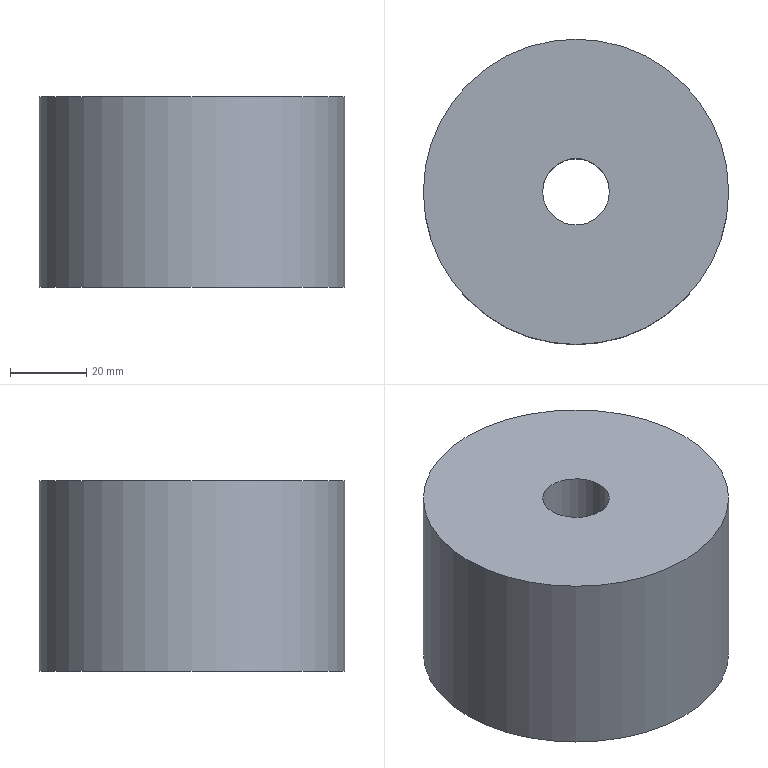Part | NX | features solid 2 | 1 solid | 4 faces | box 80 x 80 x 50 mm | volume 239301 mm3 | cylinder 2 | plane 2 | commonest cylinder face diameters 17.5 x1 80 x1
STEP:
#1=CARTESIAN_POINT('',(-1213.75,-505.,-20.));
#2=VERTEX_POINT('',#1);
#3=CARTESIAN_POINT('',(-1205.,-505.,-20.));
#4=DIRECTION('',(0.,0.,1.));
#5=DIRECTION('',(-1.,0.,0.));
#6=AXIS2_PLACEMENT_3D('',#3,#4,#5);
#7=CIRCLE('',#6,8.75);
#8=EDGE_CURVE('',#2,#2,#7,.T.);
#9=ORIENTED_EDGE('',*,*,#8,.F.);
#10=EDGE_LOOP('',(#9));
#11=FACE_BOUND('',#10,.T.);
#12=CARTESIAN_POINT('',(-1213.75,-505.,30.));
#13=VERTEX_POINT('',#12);
#14=CARTESIAN_POINT('',(-1205.,-505.,30.));
#15=DIRECTION('',(0.,0.,1.));
#16=DIRECTION('',(-1.,0.,0.));
#17=AXIS2_PLACEMENT_3D('',#14,#15,#16);
#18=CIRCLE('',#17,8.75);
#19=EDGE_CURVE('',#13,#13,#18,.T.);
#20=ORIENTED_EDGE('',*,*,#19,.T.);
#21=EDGE_LOOP('',(#20));
#22=FACE_BOUND('',#21,.T.);
#23=CARTESIAN_POINT('',(-1205.,-505.,-20.));
#24=DIRECTION('',(0.,0.,1.));
#25=DIRECTION('',(1.,0.,0.));
#26=AXIS2_PLACEMENT_3D('',#23,#24,#25);
#27=CYLINDRICAL_SURFACE('',#26,8.75);
#28=ADVANCED_FACE('',(#11,#22),#27,.F.);
#29=CARTESIAN_POINT('',(-1245.,-505.,-20.));
#30=VERTEX_POINT('',#29);
#31=CARTESIAN_POINT('',(-1205.,-505.,-20.));
#32=DIRECTION('',(0.,0.,1.));
#33=DIRECTION('',(-1.,0.,0.));
#34=AXIS2_PLACEMENT_3D('',#31,#32,#33);
#35=CIRCLE('',#34,40.);
#36=EDGE_CURVE('',#30,#30,#35,.T.);
#37=ORIENTED_EDGE('',*,*,#36,.T.);
#38=EDGE_LOOP('',(#37));
#39=FACE_BOUND('',#38,.T.);
#40=CARTESIAN_POINT('',(-1245.,-505.,30.));
#41=VERTEX_POINT('',#40);
#42=CARTESIAN_POINT('',(-1205.,-505.,30.));
#43=DIRECTION('',(0.,0.,1.));
#44=DIRECTION('',(-1.,0.,0.));
#45=AXIS2_PLACEMENT_3D('',#42,#43,#44);
#46=CIRCLE('',#45,40.);
#47=EDGE_CURVE('',#41,#41,#46,.T.);
#48=ORIENTED_EDGE('',*,*,#47,.F.);
#49=EDGE_LOOP('',(#48));
#50=FACE_BOUND('',#49,.T.);
#51=CARTESIAN_POINT('',(-1205.,-505.,-20.));
#52=DIRECTION('',(0.,0.,1.));
#53=DIRECTION('',(1.,0.,0.));
#54=AXIS2_PLACEMENT_3D('',#51,#52,#53);
#55=CYLINDRICAL_SURFACE('',#54,40.);
#56=ADVANCED_FACE('',(#39,#50),#55,.T.);
#57=ORIENTED_EDGE('',*,*,#8,.T.);
#58=EDGE_LOOP('',(#57));
#59=FACE_BOUND('',#58,.T.);
#60=ORIENTED_EDGE('',*,*,#36,.F.);
#61=EDGE_LOOP('',(#60));
#62=FACE_BOUND('',#61,.T.);
#63=CARTESIAN_POINT('',(-1205.,-505.,-20.));
#64=DIRECTION('',(0.,0.,1.));
#65=DIRECTION('',(-1.,0.,0.));
#66=AXIS2_PLACEMENT_3D('',#63,#64,#65);
#67=PLANE('',#66);
#68=ADVANCED_FACE('',(#59,#62),#67,.F.);
#69=ORIENTED_EDGE('',*,*,#19,.F.);
#70=EDGE_LOOP('',(#69));
#71=FACE_BOUND('',#70,.T.);
#72=ORIENTED_EDGE('',*,*,#47,.T.);
#73=EDGE_LOOP('',(#72));
#74=FACE_BOUND('',#73,.T.);
#75=CARTESIAN_POINT('',(-1205.,-505.,30.));
#76=DIRECTION('',(0.,0.,1.));
#77=DIRECTION('',(-1.,0.,0.));
#78=AXIS2_PLACEMENT_3D('',#75,#76,#77);
#79=PLANE('',#78);
#80=ADVANCED_FACE('',(#71,#74),#79,.T.);
#81=CLOSED_SHELL('',(#28,#56,#68,#80));
#82=MANIFOLD_SOLID_BREP('',#81);
#83=(LENGTH_UNIT()NAMED_UNIT(*)SI_UNIT(.MILLI.,.METRE.));
#84=UNCERTAINTY_MEASURE_WITH_UNIT(LENGTH_MEASURE(0.00001),#83,'','');
#85=(NAMED_UNIT(*)PLANE_ANGLE_UNIT()SI_UNIT($,.RADIAN.));
#86=(NAMED_UNIT(*)SI_UNIT($,.STERADIAN.)SOLID_ANGLE_UNIT());
#87=(GEOMETRIC_REPRESENTATION_CONTEXT(3)GLOBAL_UNCERTAINTY_ASSIGNED_CONTEXT((#84))GLOBAL_UNIT_ASSIGNED_CONTEXT((#83,#85,#86))REPRESENTATION_CONTEXT('',''));
#88=ADVANCED_BREP_SHAPE_REPRESENTATION('',(#82),#87);